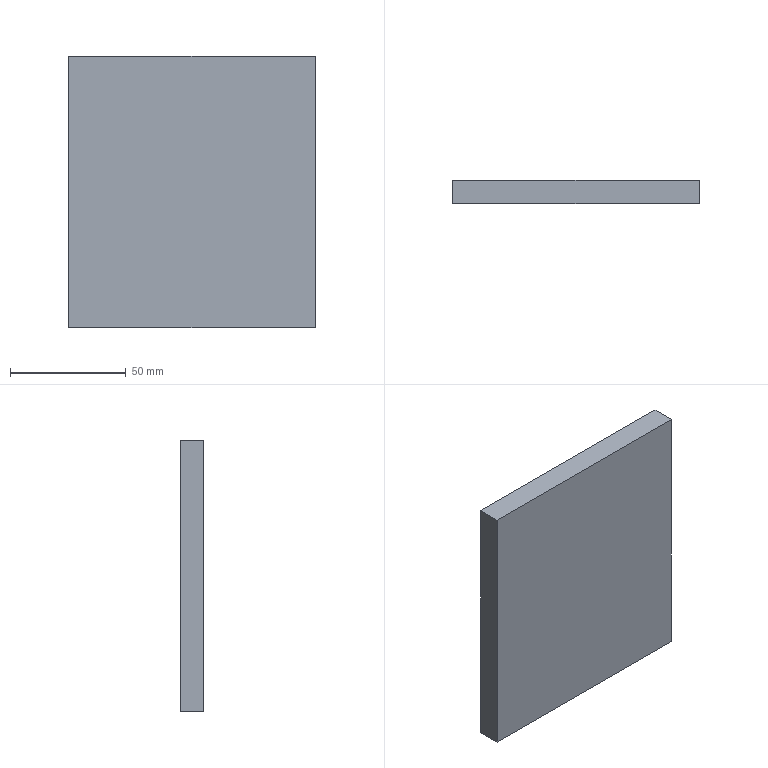Part | STEP file | 4-20.sldasm-Part-205 | 1 solid | 6 faces | box 106.7 x 10 x 117.65 mm | volume 125533 mm3 | plane 6
STEP:
#1=CARTESIAN_POINT('',(284.345,535.,-14.35));
#2=VERTEX_POINT('',#1);
#3=CARTESIAN_POINT('',(284.345,525.,-14.35));
#4=VERTEX_POINT('',#3);
#5=CARTESIAN_POINT('',(284.345,530.,-14.35));
#6=DIRECTION('',(0.,-1.,0.));
#7=VECTOR('',#6,1000.);
#8=LINE('',#5,#7);
#9=EDGE_CURVE('',#2,#4,#8,.T.);
#10=ORIENTED_EDGE('',*,*,#9,.F.);
#11=CARTESIAN_POINT('',(177.645,535.,-14.35));
#12=VERTEX_POINT('',#11);
#13=CARTESIAN_POINT('',(263.495,535.,-14.35));
#14=DIRECTION('',(1.,0.,0.));
#15=VECTOR('',#14,1000.);
#16=LINE('',#13,#15);
#17=EDGE_CURVE('',#12,#2,#16,.T.);
#18=ORIENTED_EDGE('',*,*,#17,.F.);
#19=CARTESIAN_POINT('',(177.645,525.,-14.35));
#20=VERTEX_POINT('',#19);
#21=CARTESIAN_POINT('',(177.645,530.,-14.35));
#22=DIRECTION('',(0.,1.,0.));
#23=VECTOR('',#22,1000.);
#24=LINE('',#21,#23);
#25=EDGE_CURVE('',#20,#12,#24,.T.);
#26=ORIENTED_EDGE('',*,*,#25,.F.);
#27=CARTESIAN_POINT('',(263.495,525.,-14.35));
#28=DIRECTION('',(-1.,0.,0.));
#29=VECTOR('',#28,1000.);
#30=LINE('',#27,#29);
#31=EDGE_CURVE('',#4,#20,#30,.T.);
#32=ORIENTED_EDGE('',*,*,#31,.F.);
#33=EDGE_LOOP('',(#10,#18,#26,#32));
#34=FACE_OUTER_BOUND('',#33,.T.);
#35=CARTESIAN_POINT('',(263.495,530.,-14.35));
#36=DIRECTION('',(0.,0.,1.));
#37=DIRECTION('',(0.,1.,0.));
#38=AXIS2_PLACEMENT_3D('',#35,#36,#37);
#39=PLANE('',#38);
#40=ADVANCED_FACE('',(#34),#39,.T.);
#41=CARTESIAN_POINT('',(284.345,535.,-132.));
#42=VERTEX_POINT('',#41);
#43=CARTESIAN_POINT('',(284.345,535.,-98.65));
#44=DIRECTION('',(0.,0.,1.));
#45=VECTOR('',#44,1000.);
#46=LINE('',#43,#45);
#47=EDGE_CURVE('',#42,#2,#46,.T.);
#48=ORIENTED_EDGE('',*,*,#47,.T.);
#49=ORIENTED_EDGE('',*,*,#9,.T.);
#50=CARTESIAN_POINT('',(284.345,525.,-132.));
#51=VERTEX_POINT('',#50);
#52=CARTESIAN_POINT('',(284.345,525.,-98.65));
#53=DIRECTION('',(0.,0.,1.));
#54=VECTOR('',#53,1000.);
#55=LINE('',#52,#54);
#56=EDGE_CURVE('',#51,#4,#55,.T.);
#57=ORIENTED_EDGE('',*,*,#56,.F.);
#58=CARTESIAN_POINT('',(284.345,530.,-132.));
#59=DIRECTION('',(0.,1.,0.));
#60=VECTOR('',#59,1000.);
#61=LINE('',#58,#60);
#62=EDGE_CURVE('',#51,#42,#61,.T.);
#63=ORIENTED_EDGE('',*,*,#62,.T.);
#64=EDGE_LOOP('',(#48,#49,#57,#63));
#65=FACE_OUTER_BOUND('',#64,.T.);
#66=CARTESIAN_POINT('',(284.345,530.,-98.65));
#67=DIRECTION('',(1.,0.,0.));
#68=DIRECTION('',(0.,0.,-1.));
#69=AXIS2_PLACEMENT_3D('',#66,#67,#68);
#70=PLANE('',#69);
#71=ADVANCED_FACE('',(#65),#70,.T.);
#72=ORIENTED_EDGE('',*,*,#56,.T.);
#73=ORIENTED_EDGE('',*,*,#31,.T.);
#74=CARTESIAN_POINT('',(177.645,525.,-132.));
#75=VERTEX_POINT('',#74);
#76=CARTESIAN_POINT('',(177.645,525.,-98.65));
#77=DIRECTION('',(0.,0.,1.));
#78=VECTOR('',#77,1000.);
#79=LINE('',#76,#78);
#80=EDGE_CURVE('',#75,#20,#79,.T.);
#81=ORIENTED_EDGE('',*,*,#80,.F.);
#82=CARTESIAN_POINT('',(263.495,525.,-132.));
#83=DIRECTION('',(1.,0.,0.));
#84=VECTOR('',#83,1000.);
#85=LINE('',#82,#84);
#86=EDGE_CURVE('',#75,#51,#85,.T.);
#87=ORIENTED_EDGE('',*,*,#86,.T.);
#88=EDGE_LOOP('',(#72,#73,#81,#87));
#89=FACE_OUTER_BOUND('',#88,.T.);
#90=CARTESIAN_POINT('',(263.495,525.,-98.65));
#91=DIRECTION('',(0.,-1.,0.));
#92=DIRECTION('',(0.,0.,1.));
#93=AXIS2_PLACEMENT_3D('',#90,#91,#92);
#94=PLANE('',#93);
#95=ADVANCED_FACE('',(#89),#94,.T.);
#96=ORIENTED_EDGE('',*,*,#80,.T.);
#97=ORIENTED_EDGE('',*,*,#25,.T.);
#98=CARTESIAN_POINT('',(177.645,535.,-132.));
#99=VERTEX_POINT('',#98);
#100=CARTESIAN_POINT('',(177.645,535.,-98.65));
#101=DIRECTION('',(0.,0.,1.));
#102=VECTOR('',#101,1000.);
#103=LINE('',#100,#102);
#104=EDGE_CURVE('',#99,#12,#103,.T.);
#105=ORIENTED_EDGE('',*,*,#104,.F.);
#106=CARTESIAN_POINT('',(177.645,530.,-132.));
#107=DIRECTION('',(0.,-1.,0.));
#108=VECTOR('',#107,1000.);
#109=LINE('',#106,#108);
#110=EDGE_CURVE('',#99,#75,#109,.T.);
#111=ORIENTED_EDGE('',*,*,#110,.T.);
#112=EDGE_LOOP('',(#96,#97,#105,#111));
#113=FACE_OUTER_BOUND('',#112,.T.);
#114=CARTESIAN_POINT('',(177.645,530.,-98.65));
#115=DIRECTION('',(-1.,0.,0.));
#116=DIRECTION('',(0.,0.,1.));
#117=AXIS2_PLACEMENT_3D('',#114,#115,#116);
#118=PLANE('',#117);
#119=ADVANCED_FACE('',(#113),#118,.T.);
#120=CARTESIAN_POINT('',(263.495,535.,-132.));
#121=DIRECTION('',(-1.,0.,0.));
#122=VECTOR('',#121,1000.);
#123=LINE('',#120,#122);
#124=EDGE_CURVE('',#42,#99,#123,.T.);
#125=ORIENTED_EDGE('',*,*,#124,.F.);
#126=ORIENTED_EDGE('',*,*,#62,.F.);
#127=ORIENTED_EDGE('',*,*,#86,.F.);
#128=ORIENTED_EDGE('',*,*,#110,.F.);
#129=EDGE_LOOP('',(#125,#126,#127,#128));
#130=FACE_OUTER_BOUND('',#129,.T.);
#131=CARTESIAN_POINT('',(-326.785,-666.7,-132.));
#132=DIRECTION('',(0.,0.,-1.));
#133=DIRECTION('',(0.,1.,0.));
#134=AXIS2_PLACEMENT_3D('',#131,#132,#133);
#135=PLANE('',#134);
#136=ADVANCED_FACE('',(#130),#135,.T.);
#137=ORIENTED_EDGE('',*,*,#124,.T.);
#138=ORIENTED_EDGE('',*,*,#104,.T.);
#139=ORIENTED_EDGE('',*,*,#17,.T.);
#140=ORIENTED_EDGE('',*,*,#47,.F.);
#141=EDGE_LOOP('',(#137,#138,#139,#140));
#142=FACE_OUTER_BOUND('',#141,.T.);
#143=CARTESIAN_POINT('',(263.495,535.,-98.65));
#144=DIRECTION('',(0.,1.,0.));
#145=DIRECTION('',(0.,0.,-1.));
#146=AXIS2_PLACEMENT_3D('',#143,#144,#145);
#147=PLANE('',#146);
#148=ADVANCED_FACE('',(#142),#147,.T.);
#149=CLOSED_SHELL('',(#40,#71,#95,#119,#136,#148));
#150=MANIFOLD_SOLID_BREP('',#149);
#151=CARTESIAN_POINT('',(0.,0.,0.));
#152=DIRECTION('',(0.,0.,1.));
#153=DIRECTION('',(1.,0.,0.));
#154=AXIS2_PLACEMENT_3D('',#151,#152,#153);
#155=(LENGTH_UNIT()NAMED_UNIT(*)SI_UNIT(.MILLI.,.METRE.));
#156=UNCERTAINTY_MEASURE_WITH_UNIT(LENGTH_MEASURE(0.00001),#155,'','');
#157=(NAMED_UNIT(*)PLANE_ANGLE_UNIT()SI_UNIT($,.RADIAN.));
#158=(NAMED_UNIT(*)SI_UNIT($,.STERADIAN.)SOLID_ANGLE_UNIT());
#159=(GEOMETRIC_REPRESENTATION_CONTEXT(3)GLOBAL_UNCERTAINTY_ASSIGNED_CONTEXT((#156))GLOBAL_UNIT_ASSIGNED_CONTEXT((#155,#157,#158))REPRESENTATION_CONTEXT('',''));
#160=ADVANCED_BREP_SHAPE_REPRESENTATION('',(#150,#154),#159);